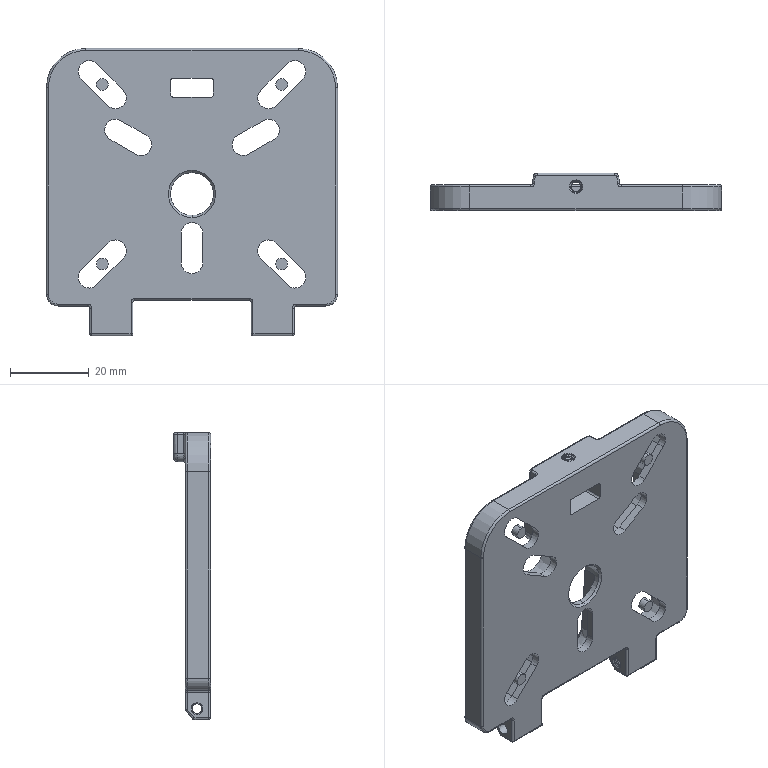Part | STEP file | DIZUO-1^M4Y_Top cover | 5 solids | 332 faces | box 74 x 9.5 x 73 mm | volume 25864 mm3 | cylinder 168 | plane 70 | spline 34 | cone 30 | torus 18 | sphere 12 | commonest cylinder face diameters 2.5 x74 1 x55 5.5 x20 3 x10 2 x3 4 x2